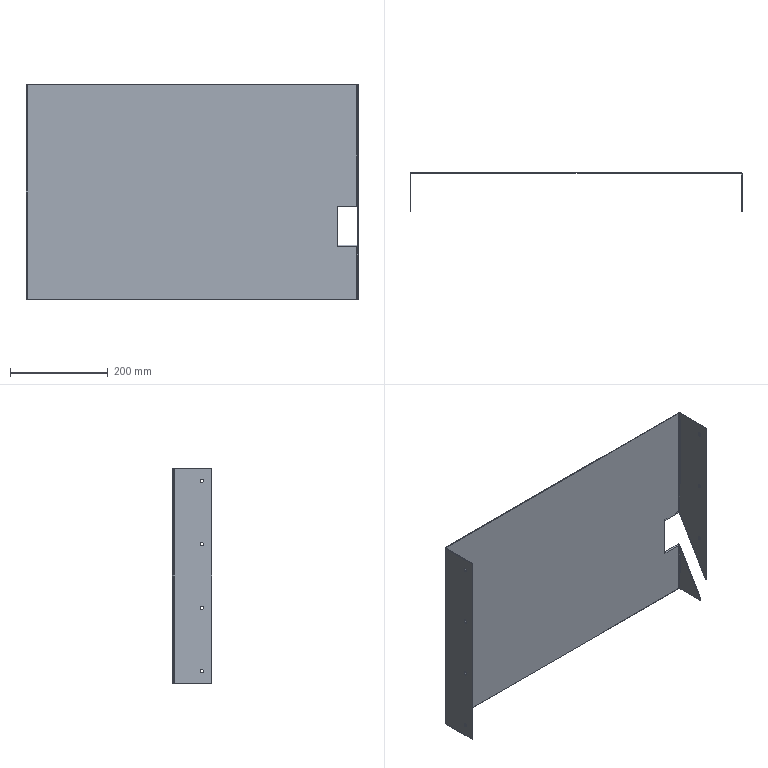Part | STEP file | C4 | 1 solid | 30 faces | box 680 x 80 x 440 mm | volume 536518 mm3 | cylinder 15 | plane 15 | commonest cylinder face diameters 7 x7 4 x5 6 x3